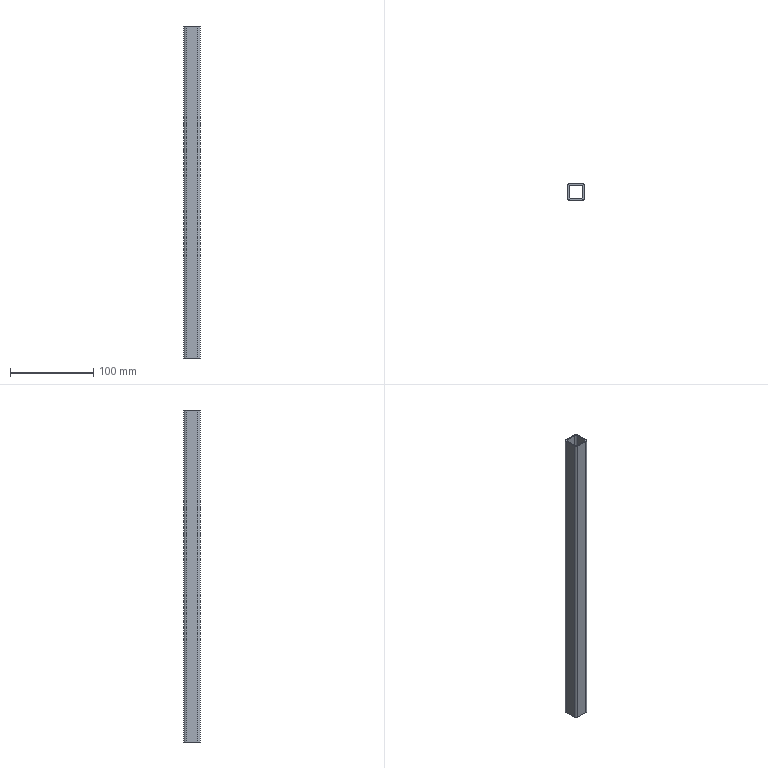Part | STEP file | DIN EN 10210-2 - 20 x 20 x 2 - 400 | 1 solid | 18 faces | box 20 x 20 x 400 mm | volume 55883 mm3 | plane 10 | cylinder 8 | commonest cylinder face diameters 4 x4 6 x4
STEP:
#1=CARTESIAN_POINT('',(0.,0.,0.));
#2=DIRECTION('',(0.,0.,1.));
#3=DIRECTION('',(1.,0.,0.));
#4=AXIS2_PLACEMENT_3D('',#1,#2,#3);
#5=CARTESIAN_POINT('',(8.,6.,0.));
#6=VERTEX_POINT('',#5);
#7=CARTESIAN_POINT('',(8.,6.,400.));
#8=VERTEX_POINT('',#7);
#9=CARTESIAN_POINT('',(8.,6.,0.));
#10=DIRECTION('',(0.,0.,1.));
#11=VECTOR('',#10,1.);
#12=LINE('',#9,#11);
#13=CARTESIAN_POINT('',(6.,6.,0.));
#14=DIRECTION('',(0.,0.,1.));
#15=DIRECTION('',(1.,0.,0.));
#16=AXIS2_PLACEMENT_3D('',#13,#14,#15);
#17=CYLINDRICAL_SURFACE('',#16,2.);
#18=CARTESIAN_POINT('',(0.,0.));
#19=DIRECTION('',(0.,1.));
#20=VECTOR('',#19,1.);
#21=LINE('',#18,#20);
#22=(GEOMETRIC_REPRESENTATION_CONTEXT(2)PARAMETRIC_REPRESENTATION_CONTEXT()REPRESENTATION_CONTEXT('',''));
#23=DEFINITIONAL_REPRESENTATION('',(#21),#22);
#24=PCURVE('',#17,#23);
#25=CARTESIAN_POINT('',(8.,6.,0.));
#26=DIRECTION('',(1.,0.,0.));
#27=DIRECTION('',(0.,0.,-1.));
#28=AXIS2_PLACEMENT_3D('',#25,#26,#27);
#29=PLANE('',#28);
#30=CARTESIAN_POINT('',(0.,0.));
#31=DIRECTION('',(-1.,0.));
#32=VECTOR('',#31,1.);
#33=LINE('',#30,#32);
#34=(GEOMETRIC_REPRESENTATION_CONTEXT(2)PARAMETRIC_REPRESENTATION_CONTEXT()REPRESENTATION_CONTEXT('',''));
#35=DEFINITIONAL_REPRESENTATION('',(#33),#34);
#36=PCURVE('',#29,#35);
#37=SURFACE_CURVE('',#12,(#24,#36),.PCURVE_S1.);
#38=EDGE_CURVE('',#6,#8,#37,.T.);
#39=ORIENTED_EDGE('',*,*,#38,.F.);
#40=CARTESIAN_POINT('',(6.,8.,0.));
#41=VERTEX_POINT('',#40);
#42=CARTESIAN_POINT('',(6.,6.,0.));
#43=DIRECTION('',(0.,0.,1.));
#44=DIRECTION('',(1.,0.,0.));
#45=AXIS2_PLACEMENT_3D('',#42,#43,#44);
#46=CIRCLE('',#45,2.);
#47=CARTESIAN_POINT('',(0.,0.));
#48=DIRECTION('',(1.,0.));
#49=VECTOR('',#48,1.);
#50=LINE('',#47,#49);
#51=(GEOMETRIC_REPRESENTATION_CONTEXT(2)PARAMETRIC_REPRESENTATION_CONTEXT()REPRESENTATION_CONTEXT('',''));
#52=DEFINITIONAL_REPRESENTATION('',(#50),#51);
#53=PCURVE('',#17,#52);
#54=CARTESIAN_POINT('',(0.,0.,0.));
#55=DIRECTION('',(0.,0.,1.));
#56=DIRECTION('',(1.,0.,0.));
#57=AXIS2_PLACEMENT_3D('',#54,#55,#56);
#58=PLANE('',#57);
#59=CARTESIAN_POINT('',(6.,6.));
#60=DIRECTION('',(1.,0.));
#61=AXIS2_PLACEMENT_2D('',#59,#60);
#62=CIRCLE('',#61,2.);
#63=(GEOMETRIC_REPRESENTATION_CONTEXT(2)PARAMETRIC_REPRESENTATION_CONTEXT()REPRESENTATION_CONTEXT('',''));
#64=DEFINITIONAL_REPRESENTATION('',(#62),#63);
#65=PCURVE('',#58,#64);
#66=SURFACE_CURVE('',#46,(#53,#65),.PCURVE_S1.);
#67=EDGE_CURVE('',#6,#41,#66,.T.);
#68=ORIENTED_EDGE('',*,*,#67,.T.);
#69=CARTESIAN_POINT('',(6.,8.,400.));
#70=VERTEX_POINT('',#69);
#71=CARTESIAN_POINT('',(6.,8.,0.));
#72=DIRECTION('',(0.,0.,1.));
#73=VECTOR('',#72,1.);
#74=LINE('',#71,#73);
#75=CARTESIAN_POINT('',(1.571,0.));
#76=DIRECTION('',(0.,1.));
#77=VECTOR('',#76,1.);
#78=LINE('',#75,#77);
#79=(GEOMETRIC_REPRESENTATION_CONTEXT(2)PARAMETRIC_REPRESENTATION_CONTEXT()REPRESENTATION_CONTEXT('',''));
#80=DEFINITIONAL_REPRESENTATION('',(#78),#79);
#81=PCURVE('',#17,#80);
#82=CARTESIAN_POINT('',(-6.,8.,0.));
#83=DIRECTION('',(0.,1.,0.));
#84=DIRECTION('',(0.,0.,1.));
#85=AXIS2_PLACEMENT_3D('',#82,#83,#84);
#86=PLANE('',#85);
#87=CARTESIAN_POINT('',(0.,12.));
#88=DIRECTION('',(1.,0.));
#89=VECTOR('',#88,1.);
#90=LINE('',#87,#89);
#91=(GEOMETRIC_REPRESENTATION_CONTEXT(2)PARAMETRIC_REPRESENTATION_CONTEXT()REPRESENTATION_CONTEXT('',''));
#92=DEFINITIONAL_REPRESENTATION('',(#90),#91);
#93=PCURVE('',#86,#92);
#94=SURFACE_CURVE('',#74,(#81,#93),.PCURVE_S1.);
#95=EDGE_CURVE('',#41,#70,#94,.T.);
#96=ORIENTED_EDGE('',*,*,#95,.T.);
#97=CARTESIAN_POINT('',(6.,6.,400.));
#98=DIRECTION('',(0.,0.,1.));
#99=DIRECTION('',(1.,0.,0.));
#100=AXIS2_PLACEMENT_3D('',#97,#98,#99);
#101=CIRCLE('',#100,2.);
#102=CARTESIAN_POINT('',(0.,400.));
#103=DIRECTION('',(1.,0.));
#104=VECTOR('',#103,1.);
#105=LINE('',#102,#104);
#106=(GEOMETRIC_REPRESENTATION_CONTEXT(2)PARAMETRIC_REPRESENTATION_CONTEXT()REPRESENTATION_CONTEXT('',''));
#107=DEFINITIONAL_REPRESENTATION('',(#105),#106);
#108=PCURVE('',#17,#107);
#109=CARTESIAN_POINT('',(0.,0.,400.));
#110=DIRECTION('',(0.,0.,1.));
#111=DIRECTION('',(1.,0.,0.));
#112=AXIS2_PLACEMENT_3D('',#109,#110,#111);
#113=PLANE('',#112);
#114=CARTESIAN_POINT('',(6.,6.));
#115=DIRECTION('',(1.,0.));
#116=AXIS2_PLACEMENT_2D('',#114,#115);
#117=CIRCLE('',#116,2.);
#118=(GEOMETRIC_REPRESENTATION_CONTEXT(2)PARAMETRIC_REPRESENTATION_CONTEXT()REPRESENTATION_CONTEXT('',''));
#119=DEFINITIONAL_REPRESENTATION('',(#117),#118);
#120=PCURVE('',#113,#119);
#121=SURFACE_CURVE('',#101,(#108,#120),.PCURVE_S1.);
#122=EDGE_CURVE('',#8,#70,#121,.T.);
#123=ORIENTED_EDGE('',*,*,#122,.F.);
#124=EDGE_LOOP('',(#39,#68,#96,#123));
#125=FACE_BOUND('',#124,.F.);
#126=ADVANCED_FACE('',(#125),#17,.F.);
#127=CARTESIAN_POINT('',(-6.,8.,400.));
#128=VERTEX_POINT('',#127);
#129=CARTESIAN_POINT('',(-3.,8.,400.));
#130=DIRECTION('',(-1.,0.,0.));
#131=VECTOR('',#130,1.);
#132=LINE('',#129,#131);
#133=CARTESIAN_POINT('',(400.,3.));
#134=DIRECTION('',(0.,-1.));
#135=VECTOR('',#134,1.);
#136=LINE('',#133,#135);
#137=(GEOMETRIC_REPRESENTATION_CONTEXT(2)PARAMETRIC_REPRESENTATION_CONTEXT()REPRESENTATION_CONTEXT('',''));
#138=DEFINITIONAL_REPRESENTATION('',(#136),#137);
#139=PCURVE('',#86,#138);
#140=CARTESIAN_POINT('',(-3.,8.));
#141=DIRECTION('',(-1.,0.));
#142=VECTOR('',#141,1.);
#143=LINE('',#140,#142);
#144=(GEOMETRIC_REPRESENTATION_CONTEXT(2)PARAMETRIC_REPRESENTATION_CONTEXT()REPRESENTATION_CONTEXT('',''));
#145=DEFINITIONAL_REPRESENTATION('',(#143),#144);
#146=PCURVE('',#113,#145);
#147=SURFACE_CURVE('',#132,(#139,#146),.PCURVE_S1.);
#148=EDGE_CURVE('',#70,#128,#147,.T.);
#149=ORIENTED_EDGE('',*,*,#148,.T.);
#150=CARTESIAN_POINT('',(-6.,8.,0.));
#151=VERTEX_POINT('',#150);
#152=CARTESIAN_POINT('',(-6.,8.,0.));
#153=DIRECTION('',(0.,0.,1.));
#154=VECTOR('',#153,1.);
#155=LINE('',#152,#154);
#156=CARTESIAN_POINT('',(0.,0.));
#157=DIRECTION('',(1.,0.));
#158=VECTOR('',#157,1.);
#159=LINE('',#156,#158);
#160=(GEOMETRIC_REPRESENTATION_CONTEXT(2)PARAMETRIC_REPRESENTATION_CONTEXT()REPRESENTATION_CONTEXT('',''));
#161=DEFINITIONAL_REPRESENTATION('',(#159),#160);
#162=PCURVE('',#86,#161);
#163=CARTESIAN_POINT('',(-6.,6.,0.));
#164=DIRECTION('',(0.,0.,1.));
#165=DIRECTION('',(0.,1.,0.));
#166=AXIS2_PLACEMENT_3D('',#163,#164,#165);
#167=CYLINDRICAL_SURFACE('',#166,2.);
#168=CARTESIAN_POINT('',(0.,0.));
#169=DIRECTION('',(0.,1.));
#170=VECTOR('',#169,1.);
#171=LINE('',#168,#170);
#172=(GEOMETRIC_REPRESENTATION_CONTEXT(2)PARAMETRIC_REPRESENTATION_CONTEXT()REPRESENTATION_CONTEXT('',''));
#173=DEFINITIONAL_REPRESENTATION('',(#171),#172);
#174=PCURVE('',#167,#173);
#175=SURFACE_CURVE('',#155,(#162,#174),.PCURVE_S1.);
#176=EDGE_CURVE('',#151,#128,#175,.T.);
#177=ORIENTED_EDGE('',*,*,#176,.F.);
#178=CARTESIAN_POINT('',(-3.,8.,0.));
#179=DIRECTION('',(-1.,0.,0.));
#180=VECTOR('',#179,1.);
#181=LINE('',#178,#180);
#182=CARTESIAN_POINT('',(0.,3.));
#183=DIRECTION('',(0.,-1.));
#184=VECTOR('',#183,1.);
#185=LINE('',#182,#184);
#186=(GEOMETRIC_REPRESENTATION_CONTEXT(2)PARAMETRIC_REPRESENTATION_CONTEXT()REPRESENTATION_CONTEXT('',''));
#187=DEFINITIONAL_REPRESENTATION('',(#185),#186);
#188=PCURVE('',#86,#187);
#189=CARTESIAN_POINT('',(-3.,8.));
#190=DIRECTION('',(-1.,0.));
#191=VECTOR('',#190,1.);
#192=LINE('',#189,#191);
#193=(GEOMETRIC_REPRESENTATION_CONTEXT(2)PARAMETRIC_REPRESENTATION_CONTEXT()REPRESENTATION_CONTEXT('',''));
#194=DEFINITIONAL_REPRESENTATION('',(#192),#193);
#195=PCURVE('',#58,#194);
#196=SURFACE_CURVE('',#181,(#188,#195),.PCURVE_S1.);
#197=EDGE_CURVE('',#41,#151,#196,.T.);
#198=ORIENTED_EDGE('',*,*,#197,.F.);
#199=ORIENTED_EDGE('',*,*,#95,.T.);
#200=EDGE_LOOP('',(#149,#177,#198,#199));
#201=FACE_BOUND('',#200,.T.);
#202=ADVANCED_FACE('',(#201),#86,.F.);
#203=ORIENTED_EDGE('',*,*,#176,.F.);
#204=CARTESIAN_POINT('',(-8.,6.,0.));
#205=VERTEX_POINT('',#204);
#206=CARTESIAN_POINT('',(-6.,6.,0.));
#207=DIRECTION('',(0.,0.,1.));
#208=DIRECTION('',(0.,1.,0.));
#209=AXIS2_PLACEMENT_3D('',#206,#207,#208);
#210=CIRCLE('',#209,2.);
#211=CARTESIAN_POINT('',(0.,0.));
#212=DIRECTION('',(1.,0.));
#213=VECTOR('',#212,1.);
#214=LINE('',#211,#213);
#215=(GEOMETRIC_REPRESENTATION_CONTEXT(2)PARAMETRIC_REPRESENTATION_CONTEXT()REPRESENTATION_CONTEXT('',''));
#216=DEFINITIONAL_REPRESENTATION('',(#214),#215);
#217=PCURVE('',#167,#216);
#218=CARTESIAN_POINT('',(-6.,6.));
#219=DIRECTION('',(0.,1.));
#220=AXIS2_PLACEMENT_2D('',#218,#219);
#221=CIRCLE('',#220,2.);
#222=(GEOMETRIC_REPRESENTATION_CONTEXT(2)PARAMETRIC_REPRESENTATION_CONTEXT()REPRESENTATION_CONTEXT('',''));
#223=DEFINITIONAL_REPRESENTATION('',(#221),#222);
#224=PCURVE('',#58,#223);
#225=SURFACE_CURVE('',#210,(#217,#224),.PCURVE_S1.);
#226=EDGE_CURVE('',#151,#205,#225,.T.);
#227=ORIENTED_EDGE('',*,*,#226,.T.);
#228=CARTESIAN_POINT('',(-8.,6.,400.));
#229=VERTEX_POINT('',#228);
#230=CARTESIAN_POINT('',(-8.,6.,0.));
#231=DIRECTION('',(0.,0.,1.));
#232=VECTOR('',#231,1.);
#233=LINE('',#230,#232);
#234=CARTESIAN_POINT('',(1.571,0.));
#235=DIRECTION('',(0.,1.));
#236=VECTOR('',#235,1.);
#237=LINE('',#234,#236);
#238=(GEOMETRIC_REPRESENTATION_CONTEXT(2)PARAMETRIC_REPRESENTATION_CONTEXT()REPRESENTATION_CONTEXT('',''));
#239=DEFINITIONAL_REPRESENTATION('',(#237),#238);
#240=PCURVE('',#167,#239);
#241=CARTESIAN_POINT('',(-8.,-6.,0.));
#242=DIRECTION('',(-1.,0.,0.));
#243=DIRECTION('',(0.,0.,1.));
#244=AXIS2_PLACEMENT_3D('',#241,#242,#243);
#245=PLANE('',#244);
#246=CARTESIAN_POINT('',(0.,12.));
#247=DIRECTION('',(1.,0.));
#248=VECTOR('',#247,1.);
#249=LINE('',#246,#248);
#250=(GEOMETRIC_REPRESENTATION_CONTEXT(2)PARAMETRIC_REPRESENTATION_CONTEXT()REPRESENTATION_CONTEXT('',''));
#251=DEFINITIONAL_REPRESENTATION('',(#249),#250);
#252=PCURVE('',#245,#251);
#253=SURFACE_CURVE('',#233,(#240,#252),.PCURVE_S1.);
#254=EDGE_CURVE('',#205,#229,#253,.T.);
#255=ORIENTED_EDGE('',*,*,#254,.T.);
#256=CARTESIAN_POINT('',(-6.,6.,400.));
#257=DIRECTION('',(0.,0.,1.));
#258=DIRECTION('',(0.,1.,0.));
#259=AXIS2_PLACEMENT_3D('',#256,#257,#258);
#260=CIRCLE('',#259,2.);
#261=CARTESIAN_POINT('',(0.,400.));
#262=DIRECTION('',(1.,0.));
#263=VECTOR('',#262,1.);
#264=LINE('',#261,#263);
#265=(GEOMETRIC_REPRESENTATION_CONTEXT(2)PARAMETRIC_REPRESENTATION_CONTEXT()REPRESENTATION_CONTEXT('',''));
#266=DEFINITIONAL_REPRESENTATION('',(#264),#265);
#267=PCURVE('',#167,#266);
#268=CARTESIAN_POINT('',(-6.,6.));
#269=DIRECTION('',(0.,1.));
#270=AXIS2_PLACEMENT_2D('',#268,#269);
#271=CIRCLE('',#270,2.);
#272=(GEOMETRIC_REPRESENTATION_CONTEXT(2)PARAMETRIC_REPRESENTATION_CONTEXT()REPRESENTATION_CONTEXT('',''));
#273=DEFINITIONAL_REPRESENTATION('',(#271),#272);
#274=PCURVE('',#113,#273);
#275=SURFACE_CURVE('',#260,(#267,#274),.PCURVE_S1.);
#276=EDGE_CURVE('',#128,#229,#275,.T.);
#277=ORIENTED_EDGE('',*,*,#276,.F.);
#278=EDGE_LOOP('',(#203,#227,#255,#277));
#279=FACE_BOUND('',#278,.F.);
#280=ADVANCED_FACE('',(#279),#167,.F.);
#281=CARTESIAN_POINT('',(-8.,-6.,400.));
#282=VERTEX_POINT('',#281);
#283=CARTESIAN_POINT('',(-8.,-3.,400.));
#284=DIRECTION('',(0.,-1.,0.));
#285=VECTOR('',#284,1.);
#286=LINE('',#283,#285);
#287=CARTESIAN_POINT('',(400.,3.));
#288=DIRECTION('',(0.,-1.));
#289=VECTOR('',#288,1.);
#290=LINE('',#287,#289);
#291=(GEOMETRIC_REPRESENTATION_CONTEXT(2)PARAMETRIC_REPRESENTATION_CONTEXT()REPRESENTATION_CONTEXT('',''));
#292=DEFINITIONAL_REPRESENTATION('',(#290),#291);
#293=PCURVE('',#245,#292);
#294=CARTESIAN_POINT('',(-8.,-3.));
#295=DIRECTION('',(0.,-1.));
#296=VECTOR('',#295,1.);
#297=LINE('',#294,#296);
#298=(GEOMETRIC_REPRESENTATION_CONTEXT(2)PARAMETRIC_REPRESENTATION_CONTEXT()REPRESENTATION_CONTEXT('',''));
#299=DEFINITIONAL_REPRESENTATION('',(#297),#298);
#300=PCURVE('',#113,#299);
#301=SURFACE_CURVE('',#286,(#293,#300),.PCURVE_S1.);
#302=EDGE_CURVE('',#229,#282,#301,.T.);
#303=ORIENTED_EDGE('',*,*,#302,.T.);
#304=CARTESIAN_POINT('',(-8.,-6.,0.));
#305=VERTEX_POINT('',#304);
#306=CARTESIAN_POINT('',(-8.,-6.,0.));
#307=DIRECTION('',(0.,0.,1.));
#308=VECTOR('',#307,1.);
#309=LINE('',#306,#308);
#310=CARTESIAN_POINT('',(0.,0.));
#311=DIRECTION('',(1.,0.));
#312=VECTOR('',#311,1.);
#313=LINE('',#310,#312);
#314=(GEOMETRIC_REPRESENTATION_CONTEXT(2)PARAMETRIC_REPRESENTATION_CONTEXT()REPRESENTATION_CONTEXT('',''));
#315=DEFINITIONAL_REPRESENTATION('',(#313),#314);
#316=PCURVE('',#245,#315);
#317=CARTESIAN_POINT('',(-6.,-6.,0.));
#318=DIRECTION('',(0.,0.,1.));
#319=DIRECTION('',(-1.,0.,0.));
#320=AXIS2_PLACEMENT_3D('',#317,#318,#319);
#321=CYLINDRICAL_SURFACE('',#320,2.);
#322=CARTESIAN_POINT('',(0.,0.));
#323=DIRECTION('',(0.,1.));
#324=VECTOR('',#323,1.);
#325=LINE('',#322,#324);
#326=(GEOMETRIC_REPRESENTATION_CONTEXT(2)PARAMETRIC_REPRESENTATION_CONTEXT()REPRESENTATION_CONTEXT('',''));
#327=DEFINITIONAL_REPRESENTATION('',(#325),#326);
#328=PCURVE('',#321,#327);
#329=SURFACE_CURVE('',#309,(#316,#328),.PCURVE_S1.);
#330=EDGE_CURVE('',#305,#282,#329,.T.);
#331=ORIENTED_EDGE('',*,*,#330,.F.);
#332=CARTESIAN_POINT('',(-8.,-3.,0.));
#333=DIRECTION('',(0.,-1.,0.));
#334=VECTOR('',#333,1.);
#335=LINE('',#332,#334);
#336=CARTESIAN_POINT('',(0.,3.));
#337=DIRECTION('',(0.,-1.));
#338=VECTOR('',#337,1.);
#339=LINE('',#336,#338);
#340=(GEOMETRIC_REPRESENTATION_CONTEXT(2)PARAMETRIC_REPRESENTATION_CONTEXT()REPRESENTATION_CONTEXT('',''));
#341=DEFINITIONAL_REPRESENTATION('',(#339),#340);
#342=PCURVE('',#245,#341);
#343=CARTESIAN_POINT('',(-8.,-3.));
#344=DIRECTION('',(0.,-1.));
#345=VECTOR('',#344,1.);
#346=LINE('',#343,#345);
#347=(GEOMETRIC_REPRESENTATION_CONTEXT(2)PARAMETRIC_REPRESENTATION_CONTEXT()REPRESENTATION_CONTEXT('',''));
#348=DEFINITIONAL_REPRESENTATION('',(#346),#347);
#349=PCURVE('',#58,#348);
#350=SURFACE_CURVE('',#335,(#342,#349),.PCURVE_S1.);
#351=EDGE_CURVE('',#205,#305,#350,.T.);
#352=ORIENTED_EDGE('',*,*,#351,.F.);
#353=ORIENTED_EDGE('',*,*,#254,.T.);
#354=EDGE_LOOP('',(#303,#331,#352,#353));
#355=FACE_BOUND('',#354,.T.);
#356=ADVANCED_FACE('',(#355),#245,.F.);
#357=CARTESIAN_POINT('',(10.,7.,400.));
#358=VERTEX_POINT('',#357);
#359=CARTESIAN_POINT('',(10.,-7.,400.));
#360=VERTEX_POINT('',#359);
#361=CARTESIAN_POINT('',(10.,3.5,400.));
#362=DIRECTION('',(0.,-1.,0.));
#363=VECTOR('',#362,1.);
#364=LINE('',#361,#363);
#365=CARTESIAN_POINT('',(10.,7.,0.));
#366=DIRECTION('',(1.,0.,0.));
#367=DIRECTION('',(0.,0.,-1.));
#368=AXIS2_PLACEMENT_3D('',#365,#366,#367);
#369=PLANE('',#368);
#370=CARTESIAN_POINT('',(-400.,-3.5));
#371=DIRECTION('',(0.,-1.));
#372=VECTOR('',#371,1.);
#373=LINE('',#370,#372);
#374=(GEOMETRIC_REPRESENTATION_CONTEXT(2)PARAMETRIC_REPRESENTATION_CONTEXT()REPRESENTATION_CONTEXT('',''));
#375=DEFINITIONAL_REPRESENTATION('',(#373),#374);
#376=PCURVE('',#369,#375);
#377=CARTESIAN_POINT('',(10.,3.5));
#378=DIRECTION('',(0.,-1.));
#379=VECTOR('',#378,1.);
#380=LINE('',#377,#379);
#381=(GEOMETRIC_REPRESENTATION_CONTEXT(2)PARAMETRIC_REPRESENTATION_CONTEXT()REPRESENTATION_CONTEXT('',''));
#382=DEFINITIONAL_REPRESENTATION('',(#380),#381);
#383=PCURVE('',#113,#382);
#384=SURFACE_CURVE('',#364,(#376,#383),.PCURVE_S1.);
#385=EDGE_CURVE('',#358,#360,#384,.T.);
#386=ORIENTED_EDGE('',*,*,#385,.T.);
#387=CARTESIAN_POINT('',(10.,-7.,0.));
#388=VERTEX_POINT('',#387);
#389=CARTESIAN_POINT('',(10.,-7.,0.));
#390=DIRECTION('',(0.,0.,1.));
#391=VECTOR('',#390,1.);
#392=LINE('',#389,#391);
#393=CARTESIAN_POINT('',(0.,-14.));
#394=DIRECTION('',(-1.,0.));
#395=VECTOR('',#394,1.);
#396=LINE('',#393,#395);
#397=(GEOMETRIC_REPRESENTATION_CONTEXT(2)PARAMETRIC_REPRESENTATION_CONTEXT()REPRESENTATION_CONTEXT('',''));
#398=DEFINITIONAL_REPRESENTATION('',(#396),#397);
#399=PCURVE('',#369,#398);
#400=CARTESIAN_POINT('',(7.,-7.,0.));
#401=DIRECTION('',(0.,0.,1.));
#402=DIRECTION('',(0.,1.,0.));
#403=AXIS2_PLACEMENT_3D('',#400,#401,#402);
#404=CYLINDRICAL_SURFACE('',#403,3.);
#405=CARTESIAN_POINT('',(4.712,0.));
#406=DIRECTION('',(0.,1.));
#407=VECTOR('',#406,1.);
#408=LINE('',#405,#407);
#409=(GEOMETRIC_REPRESENTATION_CONTEXT(2)PARAMETRIC_REPRESENTATION_CONTEXT()REPRESENTATION_CONTEXT('',''));
#410=DEFINITIONAL_REPRESENTATION('',(#408),#409);
#411=PCURVE('',#404,#410);
#412=SURFACE_CURVE('',#392,(#399,#411),.PCURVE_S1.);
#413=EDGE_CURVE('',#388,#360,#412,.T.);
#414=ORIENTED_EDGE('',*,*,#413,.F.);
#415=CARTESIAN_POINT('',(10.,7.,0.));
#416=VERTEX_POINT('',#415);
#417=CARTESIAN_POINT('',(10.,3.5,0.));
#418=DIRECTION('',(0.,-1.,0.));
#419=VECTOR('',#418,1.);
#420=LINE('',#417,#419);
#421=CARTESIAN_POINT('',(0.,-3.5));
#422=DIRECTION('',(0.,-1.));
#423=VECTOR('',#422,1.);
#424=LINE('',#421,#423);
#425=(GEOMETRIC_REPRESENTATION_CONTEXT(2)PARAMETRIC_REPRESENTATION_CONTEXT()REPRESENTATION_CONTEXT('',''));
#426=DEFINITIONAL_REPRESENTATION('',(#424),#425);
#427=PCURVE('',#369,#426);
#428=CARTESIAN_POINT('',(10.,3.5));
#429=DIRECTION('',(0.,-1.));
#430=VECTOR('',#429,1.);
#431=LINE('',#428,#430);
#432=(GEOMETRIC_REPRESENTATION_CONTEXT(2)PARAMETRIC_REPRESENTATION_CONTEXT()REPRESENTATION_CONTEXT('',''));
#433=DEFINITIONAL_REPRESENTATION('',(#431),#432);
#434=PCURVE('',#58,#433);
#435=SURFACE_CURVE('',#420,(#427,#434),.PCURVE_S1.);
#436=EDGE_CURVE('',#416,#388,#435,.T.);
#437=ORIENTED_EDGE('',*,*,#436,.F.);
#438=CARTESIAN_POINT('',(10.,7.,0.));
#439=DIRECTION('',(0.,0.,1.));
#440=VECTOR('',#439,1.);
#441=LINE('',#438,#440);
#442=CARTESIAN_POINT('',(0.,0.));
#443=DIRECTION('',(-1.,0.));
#444=VECTOR('',#443,1.);
#445=LINE('',#442,#444);
#446=(GEOMETRIC_REPRESENTATION_CONTEXT(2)PARAMETRIC_REPRESENTATION_CONTEXT()REPRESENTATION_CONTEXT('',''));
#447=DEFINITIONAL_REPRESENTATION('',(#445),#446);
#448=PCURVE('',#369,#447);
#449=CARTESIAN_POINT('',(7.,7.,0.));
#450=DIRECTION('',(0.,0.,1.));
#451=DIRECTION('',(-1.,0.,0.));
#452=AXIS2_PLACEMENT_3D('',#449,#450,#451);
#453=CYLINDRICAL_SURFACE('',#452,3.);
#454=CARTESIAN_POINT('',(3.142,0.));
#455=DIRECTION('',(0.,1.));
#456=VECTOR('',#455,1.);
#457=LINE('',#454,#456);
#458=(GEOMETRIC_REPRESENTATION_CONTEXT(2)PARAMETRIC_REPRESENTATION_CONTEXT()REPRESENTATION_CONTEXT('',''));
#459=DEFINITIONAL_REPRESENTATION('',(#457),#458);
#460=PCURVE('',#453,#459);
#461=SURFACE_CURVE('',#441,(#448,#460),.PCURVE_S1.);
#462=EDGE_CURVE('',#416,#358,#461,.T.);
#463=ORIENTED_EDGE('',*,*,#462,.T.);
#464=EDGE_LOOP('',(#386,#414,#437,#463));
#465=FACE_BOUND('',#464,.T.);
#466=ADVANCED_FACE('',(#465),#369,.T.);
#467=CARTESIAN_POINT('',(7.,-10.,400.));
#468=VERTEX_POINT('',#467);
#469=CARTESIAN_POINT('',(7.,-7.,400.));
#470=DIRECTION('',(0.,0.,-1.));
#471=DIRECTION('',(0.,1.,0.));
#472=AXIS2_PLACEMENT_3D('',#469,#470,#471);
#473=CIRCLE('',#472,3.);
#474=CARTESIAN_POINT('',(6.283,400.));
#475=DIRECTION('',(-1.,0.));
#476=VECTOR('',#475,1.);
#477=LINE('',#474,#476);
#478=(GEOMETRIC_REPRESENTATION_CONTEXT(2)PARAMETRIC_REPRESENTATION_CONTEXT()REPRESENTATION_CONTEXT('',''));
#479=DEFINITIONAL_REPRESENTATION('',(#477),#478);
#480=PCURVE('',#404,#479);
#481=CARTESIAN_POINT('',(7.,-4.));
#482=CARTESIAN_POINT('',(12.196,-4.));
#483=CARTESIAN_POINT('',(9.598,-8.5));
#484=CARTESIAN_POINT('',(7.,-13.));
#485=CARTESIAN_POINT('',(4.402,-8.5));
#486=CARTESIAN_POINT('',(1.804,-4.));
#487=CARTESIAN_POINT('',(7.,-4.));
#488=(BOUNDED_CURVE()B_SPLINE_CURVE(2,(#481,#482,#483,#484,#485,#486,#487),.UNSPECIFIED.,.T.,.F.)B_SPLINE_CURVE_WITH_KNOTS((1,2,2,2,2,1),(-2.094,0.,2.094,4.189,6.283,8.378),.UNSPECIFIED.)CURVE()GEOMETRIC_REPRESENTATION_ITEM()RATIONAL_B_SPLINE_CURVE((1.,0.5,1.,0.5,1.,0.5,1.))REPRESENTATION_ITEM(''));
#489=(GEOMETRIC_REPRESENTATION_CONTEXT(2)PARAMETRIC_REPRESENTATION_CONTEXT()REPRESENTATION_CONTEXT('',''));
#490=DEFINITIONAL_REPRESENTATION('',(#488),#489);
#491=PCURVE('',#113,#490);
#492=SURFACE_CURVE('',#473,(#480,#491),.PCURVE_S1.);
#493=EDGE_CURVE('',#360,#468,#492,.T.);
#494=ORIENTED_EDGE('',*,*,#493,.T.);
#495=CARTESIAN_POINT('',(7.,-10.,0.));
#496=VERTEX_POINT('',#495);
#497=CARTESIAN_POINT('',(7.,-10.,0.));
#498=DIRECTION('',(0.,0.,1.));
#499=VECTOR('',#498,1.);
#500=LINE('',#497,#499);
#501=CARTESIAN_POINT('',(3.142,0.));
#502=DIRECTION('',(0.,1.));
#503=VECTOR('',#502,1.);
#504=LINE('',#501,#503);
#505=(GEOMETRIC_REPRESENTATION_CONTEXT(2)PARAMETRIC_REPRESENTATION_CONTEXT()REPRESENTATION_CONTEXT('',''));
#506=DEFINITIONAL_REPRESENTATION('',(#504),#505);
#507=PCURVE('',#404,#506);
#508=CARTESIAN_POINT('',(7.,-10.,0.));
#509=DIRECTION('',(0.,-1.,0.));
#510=DIRECTION('',(0.,0.,-1.));
#511=AXIS2_PLACEMENT_3D('',#508,#509,#510);
#512=PLANE('',#511);
#513=CARTESIAN_POINT('',(0.,0.));
#514=DIRECTION('',(-1.,0.));
#515=VECTOR('',#514,1.);
#516=LINE('',#513,#515);
#517=(GEOMETRIC_REPRESENTATION_CONTEXT(2)PARAMETRIC_REPRESENTATION_CONTEXT()REPRESENTATION_CONTEXT('',''));
#518=DEFINITIONAL_REPRESENTATION('',(#516),#517);
#519=PCURVE('',#512,#518);
#520=SURFACE_CURVE('',#500,(#507,#519),.PCURVE_S1.);
#521=EDGE_CURVE('',#496,#468,#520,.T.);
#522=ORIENTED_EDGE('',*,*,#521,.F.);
#523=CARTESIAN_POINT('',(7.,-7.,0.));
#524=DIRECTION('',(0.,0.,-1.));
#525=DIRECTION('',(0.,1.,0.));
#526=AXIS2_PLACEMENT_3D('',#523,#524,#525);
#527=CIRCLE('',#526,3.);
#528=CARTESIAN_POINT('',(6.283,0.));
#529=DIRECTION('',(-1.,0.));
#530=VECTOR('',#529,1.);
#531=LINE('',#528,#530);
#532=(GEOMETRIC_REPRESENTATION_CONTEXT(2)PARAMETRIC_REPRESENTATION_CONTEXT()REPRESENTATION_CONTEXT('',''));
#533=DEFINITIONAL_REPRESENTATION('',(#531),#532);
#534=PCURVE('',#404,#533);
#535=CARTESIAN_POINT('',(7.,-4.));
#536=CARTESIAN_POINT('',(12.196,-4.));
#537=CARTESIAN_POINT('',(9.598,-8.5));
#538=CARTESIAN_POINT('',(7.,-13.));
#539=CARTESIAN_POINT('',(4.402,-8.5));
#540=CARTESIAN_POINT('',(1.804,-4.));
#541=CARTESIAN_POINT('',(7.,-4.));
#542=(BOUNDED_CURVE()B_SPLINE_CURVE(2,(#535,#536,#537,#538,#539,#540,#541),.UNSPECIFIED.,.T.,.F.)B_SPLINE_CURVE_WITH_KNOTS((1,2,2,2,2,1),(-2.094,0.,2.094,4.189,6.283,8.378),.UNSPECIFIED.)CURVE()GEOMETRIC_REPRESENTATION_ITEM()RATIONAL_B_SPLINE_CURVE((1.,0.5,1.,0.5,1.,0.5,1.))REPRESENTATION_ITEM(''));
#543=(GEOMETRIC_REPRESENTATION_CONTEXT(2)PARAMETRIC_REPRESENTATION_CONTEXT()REPRESENTATION_CONTEXT('',''));
#544=DEFINITIONAL_REPRESENTATION('',(#542),#543);
#545=PCURVE('',#58,#544);
#546=SURFACE_CURVE('',#527,(#534,#545),.PCURVE_S1.);
#547=EDGE_CURVE('',#388,#496,#546,.T.);
#548=ORIENTED_EDGE('',*,*,#547,.F.);
#549=ORIENTED_EDGE('',*,*,#413,.T.);
#550=EDGE_LOOP('',(#494,#522,#548,#549));
#551=FACE_BOUND('',#550,.T.);
#552=ADVANCED_FACE('',(#551),#404,.T.);
#553=CARTESIAN_POINT('',(-7.,-10.,400.));
#554=VERTEX_POINT('',#553);
#555=CARTESIAN_POINT('',(3.5,-10.,400.));
#556=DIRECTION('',(-1.,0.,0.));
#557=VECTOR('',#556,1.);
#558=LINE('',#555,#557);
#559=CARTESIAN_POINT('',(-400.,-3.5));
#560=DIRECTION('',(0.,-1.));
#561=VECTOR('',#560,1.);
#562=LINE('',#559,#561);
#563=(GEOMETRIC_REPRESENTATION_CONTEXT(2)PARAMETRIC_REPRESENTATION_CONTEXT()REPRESENTATION_CONTEXT('',''));
#564=DEFINITIONAL_REPRESENTATION('',(#562),#563);
#565=PCURVE('',#512,#564);
#566=CARTESIAN_POINT('',(3.5,-10.));
#567=DIRECTION('',(-1.,0.));
#568=VECTOR('',#567,1.);
#569=LINE('',#566,#568);
#570=(GEOMETRIC_REPRESENTATION_CONTEXT(2)PARAMETRIC_REPRESENTATION_CONTEXT()REPRESENTATION_CONTEXT('',''));
#571=DEFINITIONAL_REPRESENTATION('',(#569),#570);
#572=PCURVE('',#113,#571);
#573=SURFACE_CURVE('',#558,(#565,#572),.PCURVE_S1.);
#574=EDGE_CURVE('',#468,#554,#573,.T.);
#575=ORIENTED_EDGE('',*,*,#574,.T.);
#576=CARTESIAN_POINT('',(-7.,-10.,0.));
#577=VERTEX_POINT('',#576);
#578=CARTESIAN_POINT('',(-7.,-10.,0.));
#579=DIRECTION('',(0.,0.,1.));
#580=VECTOR('',#579,1.);
#581=LINE('',#578,#580);
#582=CARTESIAN_POINT('',(0.,-14.));
#583=DIRECTION('',(-1.,0.));
#584=VECTOR('',#583,1.);
#585=LINE('',#582,#584);
#586=(GEOMETRIC_REPRESENTATION_CONTEXT(2)PARAMETRIC_REPRESENTATION_CONTEXT()REPRESENTATION_CONTEXT('',''));
#587=DEFINITIONAL_REPRESENTATION('',(#585),#586);
#588=PCURVE('',#512,#587);
#589=CARTESIAN_POINT('',(-7.,-7.,0.));
#590=DIRECTION('',(0.,0.,1.));
#591=DIRECTION('',(1.,0.,0.));
#592=AXIS2_PLACEMENT_3D('',#589,#590,#591);
#593=CYLINDRICAL_SURFACE('',#592,3.);
#594=CARTESIAN_POINT('',(4.712,0.));
#595=DIRECTION('',(0.,1.));
#596=VECTOR('',#595,1.);
#597=LINE('',#594,#596);
#598=(GEOMETRIC_REPRESENTATION_CONTEXT(2)PARAMETRIC_REPRESENTATION_CONTEXT()REPRESENTATION_CONTEXT('',''));
#599=DEFINITIONAL_REPRESENTATION('',(#597),#598);
#600=PCURVE('',#593,#599);
#601=SURFACE_CURVE('',#581,(#588,#600),.PCURVE_S1.);
#602=EDGE_CURVE('',#577,#554,#601,.T.);
#603=ORIENTED_EDGE('',*,*,#602,.F.);
#604=CARTESIAN_POINT('',(3.5,-10.,0.));
#605=DIRECTION('',(-1.,0.,0.));
#606=VECTOR('',#605,1.);
#607=LINE('',#604,#606);
#608=CARTESIAN_POINT('',(0.,-3.5));
#609=DIRECTION('',(0.,-1.));
#610=VECTOR('',#609,1.);
#611=LINE('',#608,#610);
#612=(GEOMETRIC_REPRESENTATION_CONTEXT(2)PARAMETRIC_REPRESENTATION_CONTEXT()REPRESENTATION_CONTEXT('',''));
#613=DEFINITIONAL_REPRESENTATION('',(#611),#612);
#614=PCURVE('',#512,#613);
#615=CARTESIAN_POINT('',(3.5,-10.));
#616=DIRECTION('',(-1.,0.));
#617=VECTOR('',#616,1.);
#618=LINE('',#615,#617);
#619=(GEOMETRIC_REPRESENTATION_CONTEXT(2)PARAMETRIC_REPRESENTATION_CONTEXT()REPRESENTATION_CONTEXT('',''));
#620=DEFINITIONAL_REPRESENTATION('',(#618),#619);
#621=PCURVE('',#58,#620);
#622=SURFACE_CURVE('',#607,(#614,#621),.PCURVE_S1.);
#623=EDGE_CURVE('',#496,#577,#622,.T.);
#624=ORIENTED_EDGE('',*,*,#623,.F.);
#625=ORIENTED_EDGE('',*,*,#521,.T.);
#626=EDGE_LOOP('',(#575,#603,#624,#625));
#627=FACE_BOUND('',#626,.T.);
#628=ADVANCED_FACE('',(#627),#512,.T.);
#629=CARTESIAN_POINT('',(-10.,-7.,400.));
#630=VERTEX_POINT('',#629);
#631=CARTESIAN_POINT('',(-7.,-7.,400.));
#632=DIRECTION('',(0.,0.,-1.));
#633=DIRECTION('',(1.,0.,0.));
#634=AXIS2_PLACEMENT_3D('',#631,#632,#633);
#635=CIRCLE('',#634,3.);
#636=CARTESIAN_POINT('',(6.283,400.));
#637=DIRECTION('',(-1.,0.));
#638=VECTOR('',#637,1.);
#639=LINE('',#636,#638);
#640=(GEOMETRIC_REPRESENTATION_CONTEXT(2)PARAMETRIC_REPRESENTATION_CONTEXT()REPRESENTATION_CONTEXT('',''));
#641=DEFINITIONAL_REPRESENTATION('',(#639),#640);
#642=PCURVE('',#593,#641);
#643=CARTESIAN_POINT('',(-4.,-7.));
#644=CARTESIAN_POINT('',(-4.,-12.196));
#645=CARTESIAN_POINT('',(-8.5,-9.598));
#646=CARTESIAN_POINT('',(-13.,-7.));
#647=CARTESIAN_POINT('',(-8.5,-4.402));
#648=CARTESIAN_POINT('',(-4.,-1.804));
#649=CARTESIAN_POINT('',(-4.,-7.));
#650=(BOUNDED_CURVE()B_SPLINE_CURVE(2,(#643,#644,#645,#646,#647,#648,#649),.UNSPECIFIED.,.T.,.F.)B_SPLINE_CURVE_WITH_KNOTS((1,2,2,2,2,1),(-2.094,0.,2.094,4.189,6.283,8.378),.UNSPECIFIED.)CURVE()GEOMETRIC_REPRESENTATION_ITEM()RATIONAL_B_SPLINE_CURVE((1.,0.5,1.,0.5,1.,0.5,1.))REPRESENTATION_ITEM(''));
#651=(GEOMETRIC_REPRESENTATION_CONTEXT(2)PARAMETRIC_REPRESENTATION_CONTEXT()REPRESENTATION_CONTEXT('',''));
#652=DEFINITIONAL_REPRESENTATION('',(#650),#651);
#653=PCURVE('',#113,#652);
#654=SURFACE_CURVE('',#635,(#642,#653),.PCURVE_S1.);
#655=EDGE_CURVE('',#554,#630,#654,.T.);
#656=ORIENTED_EDGE('',*,*,#655,.T.);
#657=CARTESIAN_POINT('',(-10.,-7.,0.));
#658=VERTEX_POINT('',#657);
#659=CARTESIAN_POINT('',(-10.,-7.,0.));
#660=DIRECTION('',(0.,0.,1.));
#661=VECTOR('',#660,1.);
#662=LINE('',#659,#661);
#663=CARTESIAN_POINT('',(3.142,0.));
#664=DIRECTION('',(0.,1.));
#665=VECTOR('',#664,1.);
#666=LINE('',#663,#665);
#667=(GEOMETRIC_REPRESENTATION_CONTEXT(2)PARAMETRIC_REPRESENTATION_CONTEXT()REPRESENTATION_CONTEXT('',''));
#668=DEFINITIONAL_REPRESENTATION('',(#666),#667);
#669=PCURVE('',#593,#668);
#670=CARTESIAN_POINT('',(-10.,-7.,0.));
#671=DIRECTION('',(-1.,0.,0.));
#672=DIRECTION('',(0.,0.,1.));
#673=AXIS2_PLACEMENT_3D('',#670,#671,#672);
#674=PLANE('',#673);
#675=CARTESIAN_POINT('',(0.,0.));
#676=DIRECTION('',(1.,0.));
#677=VECTOR('',#676,1.);
#678=LINE('',#675,#677);
#679=(GEOMETRIC_REPRESENTATION_CONTEXT(2)PARAMETRIC_REPRESENTATION_CONTEXT()REPRESENTATION_CONTEXT('',''));
#680=DEFINITIONAL_REPRESENTATION('',(#678),#679);
#681=PCURVE('',#674,#680);
#682=SURFACE_CURVE('',#662,(#669,#681),.PCURVE_S1.);
#683=EDGE_CURVE('',#658,#630,#682,.T.);
#684=ORIENTED_EDGE('',*,*,#683,.F.);
#685=CARTESIAN_POINT('',(-7.,-7.,0.));
#686=DIRECTION('',(0.,0.,-1.));
#687=DIRECTION('',(1.,0.,0.));
#688=AXIS2_PLACEMENT_3D('',#685,#686,#687);
#689=CIRCLE('',#688,3.);
#690=CARTESIAN_POINT('',(6.283,0.));
#691=DIRECTION('',(-1.,0.));
#692=VECTOR('',#691,1.);
#693=LINE('',#690,#692);
#694=(GEOMETRIC_REPRESENTATION_CONTEXT(2)PARAMETRIC_REPRESENTATION_CONTEXT()REPRESENTATION_CONTEXT('',''));
#695=DEFINITIONAL_REPRESENTATION('',(#693),#694);
#696=PCURVE('',#593,#695);
#697=CARTESIAN_POINT('',(-4.,-7.));
#698=CARTESIAN_POINT('',(-4.,-12.196));
#699=CARTESIAN_POINT('',(-8.5,-9.598));
#700=CARTESIAN_POINT('',(-13.,-7.));
#701=CARTESIAN_POINT('',(-8.5,-4.402));
#702=CARTESIAN_POINT('',(-4.,-1.804));
#703=CARTESIAN_POINT('',(-4.,-7.));
#704=(BOUNDED_CURVE()B_SPLINE_CURVE(2,(#697,#698,#699,#700,#701,#702,#703),.UNSPECIFIED.,.T.,.F.)B_SPLINE_CURVE_WITH_KNOTS((1,2,2,2,2,1),(-2.094,0.,2.094,4.189,6.283,8.378),.UNSPECIFIED.)CURVE()GEOMETRIC_REPRESENTATION_ITEM()RATIONAL_B_SPLINE_CURVE((1.,0.5,1.,0.5,1.,0.5,1.))REPRESENTATION_ITEM(''));
#705=(GEOMETRIC_REPRESENTATION_CONTEXT(2)PARAMETRIC_REPRESENTATION_CONTEXT()REPRESENTATION_CONTEXT('',''));
#706=DEFINITIONAL_REPRESENTATION('',(#704),#705);
#707=PCURVE('',#58,#706);
#708=SURFACE_CURVE('',#689,(#696,#707),.PCURVE_S1.);
#709=EDGE_CURVE('',#577,#658,#708,.T.);
#710=ORIENTED_EDGE('',*,*,#709,.F.);
#711=ORIENTED_EDGE('',*,*,#602,.T.);
#712=EDGE_LOOP('',(#656,#684,#710,#711));
#713=FACE_BOUND('',#712,.T.);
#714=ADVANCED_FACE('',(#713),#593,.T.);
#715=ORIENTED_EDGE('',*,*,#330,.F.);
#716=CARTESIAN_POINT('',(-6.,-8.,0.));
#717=VERTEX_POINT('',#716);
#718=CARTESIAN_POINT('',(-6.,-6.,0.));
#719=DIRECTION('',(0.,0.,1.));
#720=DIRECTION('',(-1.,0.,0.));
#721=AXIS2_PLACEMENT_3D('',#718,#719,#720);
#722=CIRCLE('',#721,2.);
#723=CARTESIAN_POINT('',(0.,0.));
#724=DIRECTION('',(1.,0.));
#725=VECTOR('',#724,1.);
#726=LINE('',#723,#725);
#727=(GEOMETRIC_REPRESENTATION_CONTEXT(2)PARAMETRIC_REPRESENTATION_CONTEXT()REPRESENTATION_CONTEXT('',''));
#728=DEFINITIONAL_REPRESENTATION('',(#726),#727);
#729=PCURVE('',#321,#728);
#730=CARTESIAN_POINT('',(-6.,-6.));
#731=DIRECTION('',(-1.,0.));
#732=AXIS2_PLACEMENT_2D('',#730,#731);
#733=CIRCLE('',#732,2.);
#734=(GEOMETRIC_REPRESENTATION_CONTEXT(2)PARAMETRIC_REPRESENTATION_CONTEXT()REPRESENTATION_CONTEXT('',''));
#735=DEFINITIONAL_REPRESENTATION('',(#733),#734);
#736=PCURVE('',#58,#735);
#737=SURFACE_CURVE('',#722,(#729,#736),.PCURVE_S1.);
#738=EDGE_CURVE('',#305,#717,#737,.T.);
#739=ORIENTED_EDGE('',*,*,#738,.T.);
#740=CARTESIAN_POINT('',(-6.,-8.,400.));
#741=VERTEX_POINT('',#740);
#742=CARTESIAN_POINT('',(-6.,-8.,0.));
#743=DIRECTION('',(0.,0.,1.));
#744=VECTOR('',#743,1.);
#745=LINE('',#742,#744);
#746=CARTESIAN_POINT('',(1.571,0.));
#747=DIRECTION('',(0.,1.));
#748=VECTOR('',#747,1.);
#749=LINE('',#746,#748);
#750=(GEOMETRIC_REPRESENTATION_CONTEXT(2)PARAMETRIC_REPRESENTATION_CONTEXT()REPRESENTATION_CONTEXT('',''));
#751=DEFINITIONAL_REPRESENTATION('',(#749),#750);
#752=PCURVE('',#321,#751);
#753=CARTESIAN_POINT('',(6.,-8.,0.));
#754=DIRECTION('',(0.,-1.,0.));
#755=DIRECTION('',(0.,0.,-1.));
#756=AXIS2_PLACEMENT_3D('',#753,#754,#755);
#757=PLANE('',#756);
#758=CARTESIAN_POINT('',(0.,-12.));
#759=DIRECTION('',(-1.,0.));
#760=VECTOR('',#759,1.);
#761=LINE('',#758,#760);
#762=(GEOMETRIC_REPRESENTATION_CONTEXT(2)PARAMETRIC_REPRESENTATION_CONTEXT()REPRESENTATION_CONTEXT('',''));
#763=DEFINITIONAL_REPRESENTATION('',(#761),#762);
#764=PCURVE('',#757,#763);
#765=SURFACE_CURVE('',#745,(#752,#764),.PCURVE_S1.);
#766=EDGE_CURVE('',#717,#741,#765,.T.);
#767=ORIENTED_EDGE('',*,*,#766,.T.);
#768=CARTESIAN_POINT('',(-6.,-6.,400.));
#769=DIRECTION('',(0.,0.,1.));
#770=DIRECTION('',(-1.,0.,0.));
#771=AXIS2_PLACEMENT_3D('',#768,#769,#770);
#772=CIRCLE('',#771,2.);
#773=CARTESIAN_POINT('',(0.,400.));
#774=DIRECTION('',(1.,0.));
#775=VECTOR('',#774,1.);
#776=LINE('',#773,#775);
#777=(GEOMETRIC_REPRESENTATION_CONTEXT(2)PARAMETRIC_REPRESENTATION_CONTEXT()REPRESENTATION_CONTEXT('',''));
#778=DEFINITIONAL_REPRESENTATION('',(#776),#777);
#779=PCURVE('',#321,#778);
#780=CARTESIAN_POINT('',(-6.,-6.));
#781=DIRECTION('',(-1.,0.));
#782=AXIS2_PLACEMENT_2D('',#780,#781);
#783=CIRCLE('',#782,2.);
#784=(GEOMETRIC_REPRESENTATION_CONTEXT(2)PARAMETRIC_REPRESENTATION_CONTEXT()REPRESENTATION_CONTEXT('',''));
#785=DEFINITIONAL_REPRESENTATION('',(#783),#784);
#786=PCURVE('',#113,#785);
#787=SURFACE_CURVE('',#772,(#779,#786),.PCURVE_S1.);
#788=EDGE_CURVE('',#282,#741,#787,.T.);
#789=ORIENTED_EDGE('',*,*,#788,.F.);
#790=EDGE_LOOP('',(#715,#739,#767,#789));
#791=FACE_BOUND('',#790,.F.);
#792=ADVANCED_FACE('',(#791),#321,.F.);
#793=CARTESIAN_POINT('',(8.,-6.,400.));
#794=VERTEX_POINT('',#793);
#795=CARTESIAN_POINT('',(8.,3.,400.));
#796=DIRECTION('',(0.,1.,0.));
#797=VECTOR('',#796,1.);
#798=LINE('',#795,#797);
#799=CARTESIAN_POINT('',(-400.,-3.));
#800=DIRECTION('',(0.,1.));
#801=VECTOR('',#800,1.);
#802=LINE('',#799,#801);
#803=(GEOMETRIC_REPRESENTATION_CONTEXT(2)PARAMETRIC_REPRESENTATION_CONTEXT()REPRESENTATION_CONTEXT('',''));
#804=DEFINITIONAL_REPRESENTATION('',(#802),#803);
#805=PCURVE('',#29,#804);
#806=CARTESIAN_POINT('',(8.,3.));
#807=DIRECTION('',(0.,1.));
#808=VECTOR('',#807,1.);
#809=LINE('',#806,#808);
#810=(GEOMETRIC_REPRESENTATION_CONTEXT(2)PARAMETRIC_REPRESENTATION_CONTEXT()REPRESENTATION_CONTEXT('',''));
#811=DEFINITIONAL_REPRESENTATION('',(#809),#810);
#812=PCURVE('',#113,#811);
#813=SURFACE_CURVE('',#798,(#805,#812),.PCURVE_S1.);
#814=EDGE_CURVE('',#794,#8,#813,.T.);
#815=ORIENTED_EDGE('',*,*,#814,.T.);
#816=ORIENTED_EDGE('',*,*,#38,.F.);
#817=CARTESIAN_POINT('',(8.,-6.,0.));
#818=VERTEX_POINT('',#817);
#819=CARTESIAN_POINT('',(8.,3.,0.));
#820=DIRECTION('',(0.,1.,0.));
#821=VECTOR('',#820,1.);
#822=LINE('',#819,#821);
#823=CARTESIAN_POINT('',(0.,-3.));
#824=DIRECTION('',(0.,1.));
#825=VECTOR('',#824,1.);
#826=LINE('',#823,#825);
#827=(GEOMETRIC_REPRESENTATION_CONTEXT(2)PARAMETRIC_REPRESENTATION_CONTEXT()REPRESENTATION_CONTEXT('',''));
#828=DEFINITIONAL_REPRESENTATION('',(#826),#827);
#829=PCURVE('',#29,#828);
#830=CARTESIAN_POINT('',(8.,3.));
#831=DIRECTION('',(0.,1.));
#832=VECTOR('',#831,1.);
#833=LINE('',#830,#832);
#834=(GEOMETRIC_REPRESENTATION_CONTEXT(2)PARAMETRIC_REPRESENTATION_CONTEXT()REPRESENTATION_CONTEXT('',''));
#835=DEFINITIONAL_REPRESENTATION('',(#833),#834);
#836=PCURVE('',#58,#835);
#837=SURFACE_CURVE('',#822,(#829,#836),.PCURVE_S1.);
#838=EDGE_CURVE('',#818,#6,#837,.T.);
#839=ORIENTED_EDGE('',*,*,#838,.F.);
#840=CARTESIAN_POINT('',(8.,-6.,0.));
#841=DIRECTION('',(0.,0.,1.));
#842=VECTOR('',#841,1.);
#843=LINE('',#840,#842);
#844=CARTESIAN_POINT('',(0.,-12.));
#845=DIRECTION('',(-1.,0.));
#846=VECTOR('',#845,1.);
#847=LINE('',#844,#846);
#848=(GEOMETRIC_REPRESENTATION_CONTEXT(2)PARAMETRIC_REPRESENTATION_CONTEXT()REPRESENTATION_CONTEXT('',''));
#849=DEFINITIONAL_REPRESENTATION('',(#847),#848);
#850=PCURVE('',#29,#849);
#851=CARTESIAN_POINT('',(6.,-6.,0.));
#852=DIRECTION('',(0.,0.,1.));
#853=DIRECTION('',(0.,-1.,0.));
#854=AXIS2_PLACEMENT_3D('',#851,#852,#853);
#855=CYLINDRICAL_SURFACE('',#854,2.);
#856=CARTESIAN_POINT('',(1.571,0.));
#857=DIRECTION('',(0.,1.));
#858=VECTOR('',#857,1.);
#859=LINE('',#856,#858);
#860=(GEOMETRIC_REPRESENTATION_CONTEXT(2)PARAMETRIC_REPRESENTATION_CONTEXT()REPRESENTATION_CONTEXT('',''));
#861=DEFINITIONAL_REPRESENTATION('',(#859),#860);
#862=PCURVE('',#855,#861);
#863=SURFACE_CURVE('',#843,(#850,#862),.PCURVE_S1.);
#864=EDGE_CURVE('',#818,#794,#863,.T.);
#865=ORIENTED_EDGE('',*,*,#864,.T.);
#866=EDGE_LOOP('',(#815,#816,#839,#865));
#867=FACE_BOUND('',#866,.T.);
#868=ADVANCED_FACE('',(#867),#29,.F.);
#869=CARTESIAN_POINT('',(6.,-8.,0.));
#870=VERTEX_POINT('',#869);
#871=CARTESIAN_POINT('',(6.,-8.,400.));
#872=VERTEX_POINT('',#871);
#873=CARTESIAN_POINT('',(6.,-8.,0.));
#874=DIRECTION('',(0.,0.,1.));
#875=VECTOR('',#874,1.);
#876=LINE('',#873,#875);
#877=CARTESIAN_POINT('',(0.,0.));
#878=DIRECTION('',(0.,1.));
#879=VECTOR('',#878,1.);
#880=LINE('',#877,#879);
#881=(GEOMETRIC_REPRESENTATION_CONTEXT(2)PARAMETRIC_REPRESENTATION_CONTEXT()REPRESENTATION_CONTEXT('',''));
#882=DEFINITIONAL_REPRESENTATION('',(#880),#881);
#883=PCURVE('',#855,#882);
#884=CARTESIAN_POINT('',(0.,0.));
#885=DIRECTION('',(-1.,0.));
#886=VECTOR('',#885,1.);
#887=LINE('',#884,#886);
#888=(GEOMETRIC_REPRESENTATION_CONTEXT(2)PARAMETRIC_REPRESENTATION_CONTEXT()REPRESENTATION_CONTEXT('',''));
#889=DEFINITIONAL_REPRESENTATION('',(#887),#888);
#890=PCURVE('',#757,#889);
#891=SURFACE_CURVE('',#876,(#883,#890),.PCURVE_S1.);
#892=EDGE_CURVE('',#870,#872,#891,.T.);
#893=ORIENTED_EDGE('',*,*,#892,.F.);
#894=CARTESIAN_POINT('',(6.,-6.,0.));
#895=DIRECTION('',(0.,0.,1.));
#896=DIRECTION('',(0.,-1.,0.));
#897=AXIS2_PLACEMENT_3D('',#894,#895,#896);
#898=CIRCLE('',#897,2.);
#899=CARTESIAN_POINT('',(0.,0.));
#900=DIRECTION('',(1.,0.));
#901=VECTOR('',#900,1.);
#902=LINE('',#899,#901);
#903=(GEOMETRIC_REPRESENTATION_CONTEXT(2)PARAMETRIC_REPRESENTATION_CONTEXT()REPRESENTATION_CONTEXT('',''));
#904=DEFINITIONAL_REPRESENTATION('',(#902),#903);
#905=PCURVE('',#855,#904);
#906=CARTESIAN_POINT('',(6.,-6.));
#907=DIRECTION('',(0.,-1.));
#908=AXIS2_PLACEMENT_2D('',#906,#907);
#909=CIRCLE('',#908,2.);
#910=(GEOMETRIC_REPRESENTATION_CONTEXT(2)PARAMETRIC_REPRESENTATION_CONTEXT()REPRESENTATION_CONTEXT('',''));
#911=DEFINITIONAL_REPRESENTATION('',(#909),#910);
#912=PCURVE('',#58,#911);
#913=SURFACE_CURVE('',#898,(#905,#912),.PCURVE_S1.);
#914=EDGE_CURVE('',#870,#818,#913,.T.);
#915=ORIENTED_EDGE('',*,*,#914,.T.);
#916=ORIENTED_EDGE('',*,*,#864,.T.);
#917=CARTESIAN_POINT('',(6.,-6.,400.));
#918=DIRECTION('',(0.,0.,1.));
#919=DIRECTION('',(0.,-1.,0.));
#920=AXIS2_PLACEMENT_3D('',#917,#918,#919);
#921=CIRCLE('',#920,2.);
#922=CARTESIAN_POINT('',(0.,400.));
#923=DIRECTION('',(1.,0.));
#924=VECTOR('',#923,1.);
#925=LINE('',#922,#924);
#926=(GEOMETRIC_REPRESENTATION_CONTEXT(2)PARAMETRIC_REPRESENTATION_CONTEXT()REPRESENTATION_CONTEXT('',''));
#927=DEFINITIONAL_REPRESENTATION('',(#925),#926);
#928=PCURVE('',#855,#927);
#929=CARTESIAN_POINT('',(6.,-6.));
#930=DIRECTION('',(0.,-1.));
#931=AXIS2_PLACEMENT_2D('',#929,#930);
#932=CIRCLE('',#931,2.);
#933=(GEOMETRIC_REPRESENTATION_CONTEXT(2)PARAMETRIC_REPRESENTATION_CONTEXT()REPRESENTATION_CONTEXT('',''));
#934=DEFINITIONAL_REPRESENTATION('',(#932),#933);
#935=PCURVE('',#113,#934);
#936=SURFACE_CURVE('',#921,(#928,#935),.PCURVE_S1.);
#937=EDGE_CURVE('',#872,#794,#936,.T.);
#938=ORIENTED_EDGE('',*,*,#937,.F.);
#939=EDGE_LOOP('',(#893,#915,#916,#938));
#940=FACE_BOUND('',#939,.F.);
#941=ADVANCED_FACE('',(#940),#855,.F.);
#942=CARTESIAN_POINT('',(3.,-8.,400.));
#943=DIRECTION('',(1.,0.,0.));
#944=VECTOR('',#943,1.);
#945=LINE('',#942,#944);
#946=CARTESIAN_POINT('',(-400.,-3.));
#947=DIRECTION('',(0.,1.));
#948=VECTOR('',#947,1.);
#949=LINE('',#946,#948);
#950=(GEOMETRIC_REPRESENTATION_CONTEXT(2)PARAMETRIC_REPRESENTATION_CONTEXT()REPRESENTATION_CONTEXT('',''));
#951=DEFINITIONAL_REPRESENTATION('',(#949),#950);
#952=PCURVE('',#757,#951);
#953=CARTESIAN_POINT('',(3.,-8.));
#954=DIRECTION('',(1.,0.));
#955=VECTOR('',#954,1.);
#956=LINE('',#953,#955);
#957=(GEOMETRIC_REPRESENTATION_CONTEXT(2)PARAMETRIC_REPRESENTATION_CONTEXT()REPRESENTATION_CONTEXT('',''));
#958=DEFINITIONAL_REPRESENTATION('',(#956),#957);
#959=PCURVE('',#113,#958);
#960=SURFACE_CURVE('',#945,(#952,#959),.PCURVE_S1.);
#961=EDGE_CURVE('',#741,#872,#960,.T.);
#962=ORIENTED_EDGE('',*,*,#961,.T.);
#963=ORIENTED_EDGE('',*,*,#892,.F.);
#964=CARTESIAN_POINT('',(3.,-8.,0.));
#965=DIRECTION('',(1.,0.,0.));
#966=VECTOR('',#965,1.);
#967=LINE('',#964,#966);
#968=CARTESIAN_POINT('',(0.,-3.));
#969=DIRECTION('',(0.,1.));
#970=VECTOR('',#969,1.);
#971=LINE('',#968,#970);
#972=(GEOMETRIC_REPRESENTATION_CONTEXT(2)PARAMETRIC_REPRESENTATION_CONTEXT()REPRESENTATION_CONTEXT('',''));
#973=DEFINITIONAL_REPRESENTATION('',(#971),#972);
#974=PCURVE('',#757,#973);
#975=CARTESIAN_POINT('',(3.,-8.));
#976=DIRECTION('',(1.,0.));
#977=VECTOR('',#976,1.);
#978=LINE('',#975,#977);
#979=(GEOMETRIC_REPRESENTATION_CONTEXT(2)PARAMETRIC_REPRESENTATION_CONTEXT()REPRESENTATION_CONTEXT('',''));
#980=DEFINITIONAL_REPRESENTATION('',(#978),#979);
#981=PCURVE('',#58,#980);
#982=SURFACE_CURVE('',#967,(#974,#981),.PCURVE_S1.);
#983=EDGE_CURVE('',#717,#870,#982,.T.);
#984=ORIENTED_EDGE('',*,*,#983,.F.);
#985=ORIENTED_EDGE('',*,*,#766,.T.);
#986=EDGE_LOOP('',(#962,#963,#984,#985));
#987=FACE_BOUND('',#986,.T.);
#988=ADVANCED_FACE('',(#987),#757,.F.);
#989=CARTESIAN_POINT('',(-10.,7.,400.));
#990=VERTEX_POINT('',#989);
#991=CARTESIAN_POINT('',(-10.,-3.5,400.));
#992=DIRECTION('',(0.,1.,0.));
#993=VECTOR('',#992,1.);
#994=LINE('',#991,#993);
#995=CARTESIAN_POINT('',(400.,3.5));
#996=DIRECTION('',(0.,1.));
#997=VECTOR('',#996,1.);
#998=LINE('',#995,#997);
#999=(GEOMETRIC_REPRESENTATION_CONTEXT(2)PARAMETRIC_REPRESENTATION_CONTEXT()REPRESENTATION_CONTEXT('',''));
#1000=DEFINITIONAL_REPRESENTATION('',(#998),#999);
#1001=PCURVE('',#674,#1000);
#1002=CARTESIAN_POINT('',(-10.,-3.5));
#1003=DIRECTION('',(0.,1.));
#1004=VECTOR('',#1003,1.);
#1005=LINE('',#1002,#1004);
#1006=(GEOMETRIC_REPRESENTATION_CONTEXT(2)PARAMETRIC_REPRESENTATION_CONTEXT()REPRESENTATION_CONTEXT('',''));
#1007=DEFINITIONAL_REPRESENTATION('',(#1005),#1006);
#1008=PCURVE('',#113,#1007);
#1009=SURFACE_CURVE('',#994,(#1001,#1008),.PCURVE_S1.);
#1010=EDGE_CURVE('',#630,#990,#1009,.T.);
#1011=ORIENTED_EDGE('',*,*,#1010,.T.);
#1012=CARTESIAN_POINT('',(-10.,7.,0.));
#1013=VERTEX_POINT('',#1012);
#1014=CARTESIAN_POINT('',(-10.,7.,0.));
#1015=DIRECTION('',(0.,0.,1.));
#1016=VECTOR('',#1015,1.);
#1017=LINE('',#1014,#1016);
#1018=CARTESIAN_POINT('',(0.,14.));
#1019=DIRECTION('',(1.,0.));
#1020=VECTOR('',#1019,1.);
#1021=LINE('',#1018,#1020);
#1022=(GEOMETRIC_REPRESENTATION_CONTEXT(2)PARAMETRIC_REPRESENTATION_CONTEXT()REPRESENTATION_CONTEXT('',''));
#1023=DEFINITIONAL_REPRESENTATION('',(#1021),#1022);
#1024=PCURVE('',#674,#1023);
#1025=CARTESIAN_POINT('',(-7.,7.,0.));
#1026=DIRECTION('',(0.,0.,1.));
#1027=DIRECTION('',(0.,-1.,0.));
#1028=AXIS2_PLACEMENT_3D('',#1025,#1026,#1027);
#1029=CYLINDRICAL_SURFACE('',#1028,3.);
#1030=CARTESIAN_POINT('',(4.712,0.));
#1031=DIRECTION('',(0.,1.));
#1032=VECTOR('',#1031,1.);
#1033=LINE('',#1030,#1032);
#1034=(GEOMETRIC_REPRESENTATION_CONTEXT(2)PARAMETRIC_REPRESENTATION_CONTEXT()REPRESENTATION_CONTEXT('',''));
#1035=DEFINITIONAL_REPRESENTATION('',(#1033),#1034);
#1036=PCURVE('',#1029,#1035);
#1037=SURFACE_CURVE('',#1017,(#1024,#1036),.PCURVE_S1.);
#1038=EDGE_CURVE('',#1013,#990,#1037,.T.);
#1039=ORIENTED_EDGE('',*,*,#1038,.F.);
#1040=CARTESIAN_POINT('',(-10.,-3.5,0.));
#1041=DIRECTION('',(0.,1.,0.));
#1042=VECTOR('',#1041,1.);
#1043=LINE('',#1040,#1042);
#1044=CARTESIAN_POINT('',(0.,3.5));
#1045=DIRECTION('',(0.,1.));
#1046=VECTOR('',#1045,1.);
#1047=LINE('',#1044,#1046);
#1048=(GEOMETRIC_REPRESENTATION_CONTEXT(2)PARAMETRIC_REPRESENTATION_CONTEXT()REPRESENTATION_CONTEXT('',''));
#1049=DEFINITIONAL_REPRESENTATION('',(#1047),#1048);
#1050=PCURVE('',#674,#1049);
#1051=CARTESIAN_POINT('',(-10.,-3.5));
#1052=DIRECTION('',(0.,1.));
#1053=VECTOR('',#1052,1.);
#1054=LINE('',#1051,#1053);
#1055=(GEOMETRIC_REPRESENTATION_CONTEXT(2)PARAMETRIC_REPRESENTATION_CONTEXT()REPRESENTATION_CONTEXT('',''));
#1056=DEFINITIONAL_REPRESENTATION('',(#1054),#1055);
#1057=PCURVE('',#58,#1056);
#1058=SURFACE_CURVE('',#1043,(#1050,#1057),.PCURVE_S1.);
#1059=EDGE_CURVE('',#658,#1013,#1058,.T.);
#1060=ORIENTED_EDGE('',*,*,#1059,.F.);
#1061=ORIENTED_EDGE('',*,*,#683,.T.);
#1062=EDGE_LOOP('',(#1011,#1039,#1060,#1061));
#1063=FACE_BOUND('',#1062,.T.);
#1064=ADVANCED_FACE('',(#1063),#674,.T.);
#1065=CARTESIAN_POINT('',(-7.,10.,400.));
#1066=VERTEX_POINT('',#1065);
#1067=CARTESIAN_POINT('',(-7.,7.,400.));
#1068=DIRECTION('',(0.,0.,-1.));
#1069=DIRECTION('',(0.,-1.,0.));
#1070=AXIS2_PLACEMENT_3D('',#1067,#1068,#1069);
#1071=CIRCLE('',#1070,3.);
#1072=CARTESIAN_POINT('',(6.283,400.));
#1073=DIRECTION('',(-1.,0.));
#1074=VECTOR('',#1073,1.);
#1075=LINE('',#1072,#1074);
#1076=(GEOMETRIC_REPRESENTATION_CONTEXT(2)PARAMETRIC_REPRESENTATION_CONTEXT()REPRESENTATION_CONTEXT('',''));
#1077=DEFINITIONAL_REPRESENTATION('',(#1075),#1076);
#1078=PCURVE('',#1029,#1077);
#1079=CARTESIAN_POINT('',(-7.,4.));
#1080=CARTESIAN_POINT('',(-12.196,4.));
#1081=CARTESIAN_POINT('',(-9.598,8.5));
#1082=CARTESIAN_POINT('',(-7.,13.));
#1083=CARTESIAN_POINT('',(-4.402,8.5));
#1084=CARTESIAN_POINT('',(-1.804,4.));
#1085=CARTESIAN_POINT('',(-7.,4.));
#1086=(BOUNDED_CURVE()B_SPLINE_CURVE(2,(#1079,#1080,#1081,#1082,#1083,#1084,#1085),.UNSPECIFIED.,.T.,.F.)B_SPLINE_CURVE_WITH_KNOTS((1,2,2,2,2,1),(-2.094,0.,2.094,4.189,6.283,8.378),.UNSPECIFIED.)CURVE()GEOMETRIC_REPRESENTATION_ITEM()RATIONAL_B_SPLINE_CURVE((1.,0.5,1.,0.5,1.,0.5,1.))REPRESENTATION_ITEM(''));
#1087=(GEOMETRIC_REPRESENTATION_CONTEXT(2)PARAMETRIC_REPRESENTATION_CONTEXT()REPRESENTATION_CONTEXT('',''));
#1088=DEFINITIONAL_REPRESENTATION('',(#1086),#1087);
#1089=PCURVE('',#113,#1088);
#1090=SURFACE_CURVE('',#1071,(#1078,#1089),.PCURVE_S1.);
#1091=EDGE_CURVE('',#990,#1066,#1090,.T.);
#1092=ORIENTED_EDGE('',*,*,#1091,.T.);
#1093=CARTESIAN_POINT('',(-7.,10.,0.));
#1094=VERTEX_POINT('',#1093);
#1095=CARTESIAN_POINT('',(-7.,10.,0.));
#1096=DIRECTION('',(0.,0.,1.));
#1097=VECTOR('',#1096,1.);
#1098=LINE('',#1095,#1097);
#1099=CARTESIAN_POINT('',(3.142,0.));
#1100=DIRECTION('',(0.,1.));
#1101=VECTOR('',#1100,1.);
#1102=LINE('',#1099,#1101);
#1103=(GEOMETRIC_REPRESENTATION_CONTEXT(2)PARAMETRIC_REPRESENTATION_CONTEXT()REPRESENTATION_CONTEXT('',''));
#1104=DEFINITIONAL_REPRESENTATION('',(#1102),#1103);
#1105=PCURVE('',#1029,#1104);
#1106=CARTESIAN_POINT('',(-7.,10.,0.));
#1107=DIRECTION('',(0.,1.,0.));
#1108=DIRECTION('',(0.,0.,1.));
#1109=AXIS2_PLACEMENT_3D('',#1106,#1107,#1108);
#1110=PLANE('',#1109);
#1111=CARTESIAN_POINT('',(0.,0.));
#1112=DIRECTION('',(1.,0.));
#1113=VECTOR('',#1112,1.);
#1114=LINE('',#1111,#1113);
#1115=(GEOMETRIC_REPRESENTATION_CONTEXT(2)PARAMETRIC_REPRESENTATION_CONTEXT()REPRESENTATION_CONTEXT('',''));
#1116=DEFINITIONAL_REPRESENTATION('',(#1114),#1115);
#1117=PCURVE('',#1110,#1116);
#1118=SURFACE_CURVE('',#1098,(#1105,#1117),.PCURVE_S1.);
#1119=EDGE_CURVE('',#1094,#1066,#1118,.T.);
#1120=ORIENTED_EDGE('',*,*,#1119,.F.);
#1121=CARTESIAN_POINT('',(-7.,7.,0.));
#1122=DIRECTION('',(0.,0.,-1.));
#1123=DIRECTION('',(0.,-1.,0.));
#1124=AXIS2_PLACEMENT_3D('',#1121,#1122,#1123);
#1125=CIRCLE('',#1124,3.);
#1126=CARTESIAN_POINT('',(6.283,0.));
#1127=DIRECTION('',(-1.,0.));
#1128=VECTOR('',#1127,1.);
#1129=LINE('',#1126,#1128);
#1130=(GEOMETRIC_REPRESENTATION_CONTEXT(2)PARAMETRIC_REPRESENTATION_CONTEXT()REPRESENTATION_CONTEXT('',''));
#1131=DEFINITIONAL_REPRESENTATION('',(#1129),#1130);
#1132=PCURVE('',#1029,#1131);
#1133=CARTESIAN_POINT('',(-7.,4.));
#1134=CARTESIAN_POINT('',(-12.196,4.));
#1135=CARTESIAN_POINT('',(-9.598,8.5));
#1136=CARTESIAN_POINT('',(-7.,13.));
#1137=CARTESIAN_POINT('',(-4.402,8.5));
#1138=CARTESIAN_POINT('',(-1.804,4.));
#1139=CARTESIAN_POINT('',(-7.,4.));
#1140=(BOUNDED_CURVE()B_SPLINE_CURVE(2,(#1133,#1134,#1135,#1136,#1137,#1138,#1139),.UNSPECIFIED.,.T.,.F.)B_SPLINE_CURVE_WITH_KNOTS((1,2,2,2,2,1),(-2.094,0.,2.094,4.189,6.283,8.378),.UNSPECIFIED.)CURVE()GEOMETRIC_REPRESENTATION_ITEM()RATIONAL_B_SPLINE_CURVE((1.,0.5,1.,0.5,1.,0.5,1.))REPRESENTATION_ITEM(''));
#1141=(GEOMETRIC_REPRESENTATION_CONTEXT(2)PARAMETRIC_REPRESENTATION_CONTEXT()REPRESENTATION_CONTEXT('',''));
#1142=DEFINITIONAL_REPRESENTATION('',(#1140),#1141);
#1143=PCURVE('',#58,#1142);
#1144=SURFACE_CURVE('',#1125,(#1132,#1143),.PCURVE_S1.);
#1145=EDGE_CURVE('',#1013,#1094,#1144,.T.);
#1146=ORIENTED_EDGE('',*,*,#1145,.F.);
#1147=ORIENTED_EDGE('',*,*,#1038,.T.);
#1148=EDGE_LOOP('',(#1092,#1120,#1146,#1147));
#1149=FACE_BOUND('',#1148,.T.);
#1150=ADVANCED_FACE('',(#1149),#1029,.T.);
#1151=CARTESIAN_POINT('',(7.,10.,400.));
#1152=VERTEX_POINT('',#1151);
#1153=CARTESIAN_POINT('',(-3.5,10.,400.));
#1154=DIRECTION('',(1.,0.,0.));
#1155=VECTOR('',#1154,1.);
#1156=LINE('',#1153,#1155);
#1157=CARTESIAN_POINT('',(400.,3.5));
#1158=DIRECTION('',(0.,1.));
#1159=VECTOR('',#1158,1.);
#1160=LINE('',#1157,#1159);
#1161=(GEOMETRIC_REPRESENTATION_CONTEXT(2)PARAMETRIC_REPRESENTATION_CONTEXT()REPRESENTATION_CONTEXT('',''));
#1162=DEFINITIONAL_REPRESENTATION('',(#1160),#1161);
#1163=PCURVE('',#1110,#1162);
#1164=CARTESIAN_POINT('',(-3.5,10.));
#1165=DIRECTION('',(1.,0.));
#1166=VECTOR('',#1165,1.);
#1167=LINE('',#1164,#1166);
#1168=(GEOMETRIC_REPRESENTATION_CONTEXT(2)PARAMETRIC_REPRESENTATION_CONTEXT()REPRESENTATION_CONTEXT('',''));
#1169=DEFINITIONAL_REPRESENTATION('',(#1167),#1168);
#1170=PCURVE('',#113,#1169);
#1171=SURFACE_CURVE('',#1156,(#1163,#1170),.PCURVE_S1.);
#1172=EDGE_CURVE('',#1066,#1152,#1171,.T.);
#1173=ORIENTED_EDGE('',*,*,#1172,.T.);
#1174=CARTESIAN_POINT('',(7.,10.,0.));
#1175=VERTEX_POINT('',#1174);
#1176=CARTESIAN_POINT('',(7.,10.,0.));
#1177=DIRECTION('',(0.,0.,1.));
#1178=VECTOR('',#1177,1.);
#1179=LINE('',#1176,#1178);
#1180=CARTESIAN_POINT('',(0.,14.));
#1181=DIRECTION('',(1.,0.));
#1182=VECTOR('',#1181,1.);
#1183=LINE('',#1180,#1182);
#1184=(GEOMETRIC_REPRESENTATION_CONTEXT(2)PARAMETRIC_REPRESENTATION_CONTEXT()REPRESENTATION_CONTEXT('',''));
#1185=DEFINITIONAL_REPRESENTATION('',(#1183),#1184);
#1186=PCURVE('',#1110,#1185);
#1187=CARTESIAN_POINT('',(4.712,0.));
#1188=DIRECTION('',(0.,1.));
#1189=VECTOR('',#1188,1.);
#1190=LINE('',#1187,#1189);
#1191=(GEOMETRIC_REPRESENTATION_CONTEXT(2)PARAMETRIC_REPRESENTATION_CONTEXT()REPRESENTATION_CONTEXT('',''));
#1192=DEFINITIONAL_REPRESENTATION('',(#1190),#1191);
#1193=PCURVE('',#453,#1192);
#1194=SURFACE_CURVE('',#1179,(#1186,#1193),.PCURVE_S1.);
#1195=EDGE_CURVE('',#1175,#1152,#1194,.T.);
#1196=ORIENTED_EDGE('',*,*,#1195,.F.);
#1197=CARTESIAN_POINT('',(-3.5,10.,0.));
#1198=DIRECTION('',(1.,0.,0.));
#1199=VECTOR('',#1198,1.);
#1200=LINE('',#1197,#1199);
#1201=CARTESIAN_POINT('',(0.,3.5));
#1202=DIRECTION('',(0.,1.));
#1203=VECTOR('',#1202,1.);
#1204=LINE('',#1201,#1203);
#1205=(GEOMETRIC_REPRESENTATION_CONTEXT(2)PARAMETRIC_REPRESENTATION_CONTEXT()REPRESENTATION_CONTEXT('',''));
#1206=DEFINITIONAL_REPRESENTATION('',(#1204),#1205);
#1207=PCURVE('',#1110,#1206);
#1208=CARTESIAN_POINT('',(-3.5,10.));
#1209=DIRECTION('',(1.,0.));
#1210=VECTOR('',#1209,1.);
#1211=LINE('',#1208,#1210);
#1212=(GEOMETRIC_REPRESENTATION_CONTEXT(2)PARAMETRIC_REPRESENTATION_CONTEXT()REPRESENTATION_CONTEXT('',''));
#1213=DEFINITIONAL_REPRESENTATION('',(#1211),#1212);
#1214=PCURVE('',#58,#1213);
#1215=SURFACE_CURVE('',#1200,(#1207,#1214),.PCURVE_S1.);
#1216=EDGE_CURVE('',#1094,#1175,#1215,.T.);
#1217=ORIENTED_EDGE('',*,*,#1216,.F.);
#1218=ORIENTED_EDGE('',*,*,#1119,.T.);
#1219=EDGE_LOOP('',(#1173,#1196,#1217,#1218));
#1220=FACE_BOUND('',#1219,.T.);
#1221=ADVANCED_FACE('',(#1220),#1110,.T.);
#1222=CARTESIAN_POINT('',(7.,7.,400.));
#1223=DIRECTION('',(0.,0.,-1.));
#1224=DIRECTION('',(-1.,0.,0.));
#1225=AXIS2_PLACEMENT_3D('',#1222,#1223,#1224);
#1226=CIRCLE('',#1225,3.);
#1227=CARTESIAN_POINT('',(6.283,400.));
#1228=DIRECTION('',(-1.,0.));
#1229=VECTOR('',#1228,1.);
#1230=LINE('',#1227,#1229);
#1231=(GEOMETRIC_REPRESENTATION_CONTEXT(2)PARAMETRIC_REPRESENTATION_CONTEXT()REPRESENTATION_CONTEXT('',''));
#1232=DEFINITIONAL_REPRESENTATION('',(#1230),#1231);
#1233=PCURVE('',#453,#1232);
#1234=CARTESIAN_POINT('',(4.,7.));
#1235=CARTESIAN_POINT('',(4.,12.196));
#1236=CARTESIAN_POINT('',(8.5,9.598));
#1237=CARTESIAN_POINT('',(13.,7.));
#1238=CARTESIAN_POINT('',(8.5,4.402));
#1239=CARTESIAN_POINT('',(4.,1.804));
#1240=CARTESIAN_POINT('',(4.,7.));
#1241=(BOUNDED_CURVE()B_SPLINE_CURVE(2,(#1234,#1235,#1236,#1237,#1238,#1239,#1240),.UNSPECIFIED.,.T.,.F.)B_SPLINE_CURVE_WITH_KNOTS((1,2,2,2,2,1),(-2.094,0.,2.094,4.189,6.283,8.378),.UNSPECIFIED.)CURVE()GEOMETRIC_REPRESENTATION_ITEM()RATIONAL_B_SPLINE_CURVE((1.,0.5,1.,0.5,1.,0.5,1.))REPRESENTATION_ITEM(''));
#1242=(GEOMETRIC_REPRESENTATION_CONTEXT(2)PARAMETRIC_REPRESENTATION_CONTEXT()REPRESENTATION_CONTEXT('',''));
#1243=DEFINITIONAL_REPRESENTATION('',(#1241),#1242);
#1244=PCURVE('',#113,#1243);
#1245=SURFACE_CURVE('',#1226,(#1233,#1244),.PCURVE_S1.);
#1246=EDGE_CURVE('',#1152,#358,#1245,.T.);
#1247=ORIENTED_EDGE('',*,*,#1246,.T.);
#1248=ORIENTED_EDGE('',*,*,#462,.F.);
#1249=CARTESIAN_POINT('',(7.,7.,0.));
#1250=DIRECTION('',(0.,0.,-1.));
#1251=DIRECTION('',(-1.,0.,0.));
#1252=AXIS2_PLACEMENT_3D('',#1249,#1250,#1251);
#1253=CIRCLE('',#1252,3.);
#1254=CARTESIAN_POINT('',(6.283,0.));
#1255=DIRECTION('',(-1.,0.));
#1256=VECTOR('',#1255,1.);
#1257=LINE('',#1254,#1256);
#1258=(GEOMETRIC_REPRESENTATION_CONTEXT(2)PARAMETRIC_REPRESENTATION_CONTEXT()REPRESENTATION_CONTEXT('',''));
#1259=DEFINITIONAL_REPRESENTATION('',(#1257),#1258);
#1260=PCURVE('',#453,#1259);
#1261=CARTESIAN_POINT('',(4.,7.));
#1262=CARTESIAN_POINT('',(4.,12.196));
#1263=CARTESIAN_POINT('',(8.5,9.598));
#1264=CARTESIAN_POINT('',(13.,7.));
#1265=CARTESIAN_POINT('',(8.5,4.402));
#1266=CARTESIAN_POINT('',(4.,1.804));
#1267=CARTESIAN_POINT('',(4.,7.));
#1268=(BOUNDED_CURVE()B_SPLINE_CURVE(2,(#1261,#1262,#1263,#1264,#1265,#1266,#1267),.UNSPECIFIED.,.T.,.F.)B_SPLINE_CURVE_WITH_KNOTS((1,2,2,2,2,1),(-2.094,0.,2.094,4.189,6.283,8.378),.UNSPECIFIED.)CURVE()GEOMETRIC_REPRESENTATION_ITEM()RATIONAL_B_SPLINE_CURVE((1.,0.5,1.,0.5,1.,0.5,1.))REPRESENTATION_ITEM(''));
#1269=(GEOMETRIC_REPRESENTATION_CONTEXT(2)PARAMETRIC_REPRESENTATION_CONTEXT()REPRESENTATION_CONTEXT('',''));
#1270=DEFINITIONAL_REPRESENTATION('',(#1268),#1269);
#1271=PCURVE('',#58,#1270);
#1272=SURFACE_CURVE('',#1253,(#1260,#1271),.PCURVE_S1.);
#1273=EDGE_CURVE('',#1175,#416,#1272,.T.);
#1274=ORIENTED_EDGE('',*,*,#1273,.F.);
#1275=ORIENTED_EDGE('',*,*,#1195,.T.);
#1276=EDGE_LOOP('',(#1247,#1248,#1274,#1275));
#1277=FACE_BOUND('',#1276,.T.);
#1278=ADVANCED_FACE('',(#1277),#453,.T.);
#1279=ORIENTED_EDGE('',*,*,#1059,.T.);
#1280=ORIENTED_EDGE('',*,*,#1145,.T.);
#1281=ORIENTED_EDGE('',*,*,#1216,.T.);
#1282=ORIENTED_EDGE('',*,*,#1273,.T.);
#1283=ORIENTED_EDGE('',*,*,#436,.T.);
#1284=ORIENTED_EDGE('',*,*,#547,.T.);
#1285=ORIENTED_EDGE('',*,*,#623,.T.);
#1286=ORIENTED_EDGE('',*,*,#709,.T.);
#1287=EDGE_LOOP('',(#1279,#1280,#1281,#1282,#1283,#1284,#1285,#1286));
#1288=FACE_BOUND('',#1287,.T.);
#1289=ORIENTED_EDGE('',*,*,#738,.T.);
#1290=ORIENTED_EDGE('',*,*,#983,.T.);
#1291=ORIENTED_EDGE('',*,*,#914,.T.);
#1292=ORIENTED_EDGE('',*,*,#838,.T.);
#1293=ORIENTED_EDGE('',*,*,#67,.T.);
#1294=ORIENTED_EDGE('',*,*,#197,.T.);
#1295=ORIENTED_EDGE('',*,*,#226,.T.);
#1296=ORIENTED_EDGE('',*,*,#351,.T.);
#1297=EDGE_LOOP('',(#1289,#1290,#1291,#1292,#1293,#1294,#1295,#1296));
#1298=FACE_BOUND('',#1297,.T.);
#1299=ADVANCED_FACE('',(#1288,#1298),#58,.F.);
#1300=ORIENTED_EDGE('',*,*,#1010,.F.);
#1301=ORIENTED_EDGE('',*,*,#655,.F.);
#1302=ORIENTED_EDGE('',*,*,#574,.F.);
#1303=ORIENTED_EDGE('',*,*,#493,.F.);
#1304=ORIENTED_EDGE('',*,*,#385,.F.);
#1305=ORIENTED_EDGE('',*,*,#1246,.F.);
#1306=ORIENTED_EDGE('',*,*,#1172,.F.);
#1307=ORIENTED_EDGE('',*,*,#1091,.F.);
#1308=EDGE_LOOP('',(#1300,#1301,#1302,#1303,#1304,#1305,#1306,#1307));
#1309=FACE_BOUND('',#1308,.T.);
#1310=ORIENTED_EDGE('',*,*,#788,.F.);
#1311=ORIENTED_EDGE('',*,*,#302,.F.);
#1312=ORIENTED_EDGE('',*,*,#276,.F.);
#1313=ORIENTED_EDGE('',*,*,#148,.F.);
#1314=ORIENTED_EDGE('',*,*,#122,.F.);
#1315=ORIENTED_EDGE('',*,*,#814,.F.);
#1316=ORIENTED_EDGE('',*,*,#937,.F.);
#1317=ORIENTED_EDGE('',*,*,#961,.F.);
#1318=EDGE_LOOP('',(#1310,#1311,#1312,#1313,#1314,#1315,#1316,#1317));
#1319=FACE_BOUND('',#1318,.T.);
#1320=ADVANCED_FACE('',(#1309,#1319),#113,.T.);
#1321=CLOSED_SHELL('',(#126,#202,#280,#356,#466,#552,#628,#714,#792,#868,#941,#988,#1064,#1150,#1221,#1278,#1299,#1320));
#1322=MANIFOLD_SOLID_BREP('',#1321);
#1323=(LENGTH_UNIT()NAMED_UNIT(*)SI_UNIT(.MILLI.,.METRE.));
#1324=UNCERTAINTY_MEASURE_WITH_UNIT(LENGTH_MEASURE(0.0000001),#1323,'','');
#1325=(NAMED_UNIT(*)PLANE_ANGLE_UNIT()SI_UNIT($,.RADIAN.));
#1326=(NAMED_UNIT(*)SI_UNIT($,.STERADIAN.)SOLID_ANGLE_UNIT());
#1327=(GEOMETRIC_REPRESENTATION_CONTEXT(3)GLOBAL_UNCERTAINTY_ASSIGNED_CONTEXT((#1324))GLOBAL_UNIT_ASSIGNED_CONTEXT((#1323,#1325,#1326))REPRESENTATION_CONTEXT('',''));
#1328=ADVANCED_BREP_SHAPE_REPRESENTATION('',(#4,#1322),#1327);